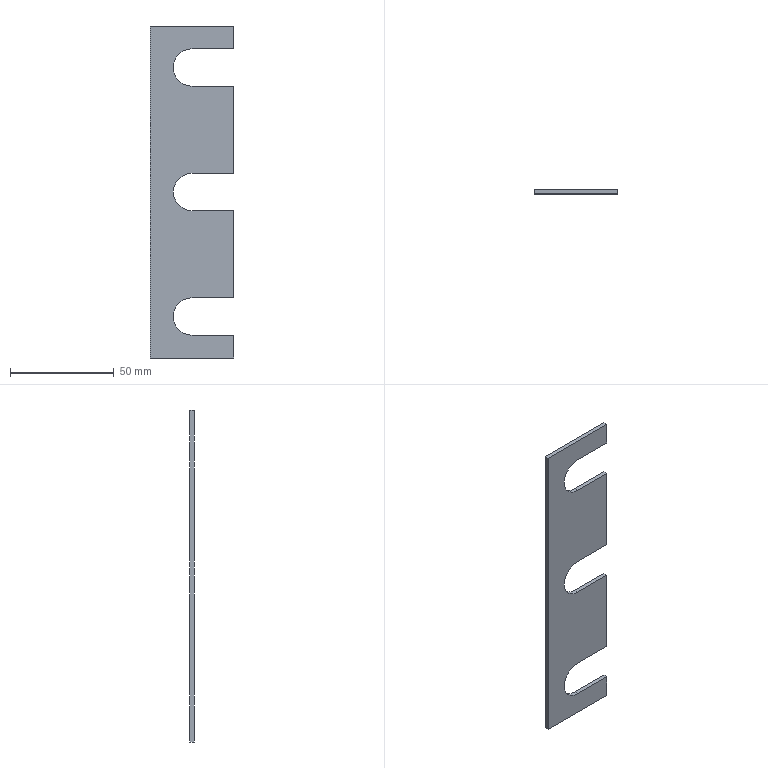Part | SolidWorks | features MirrorStock 1 | 1 solid | 18 faces | box 40 x 2 x 160 mm | volume 9877 mm3 | plane 15 | cylinder 3 | commonest cylinder face diameters 18 x3
STEP:
#1=CARTESIAN_POINT('',(0.,0.,-9.));
#2=VERTEX_POINT('',#1);
#3=CARTESIAN_POINT('',(0.,0.,9.));
#4=VERTEX_POINT('',#3);
#5=CARTESIAN_POINT('',(0.,0.,0.));
#6=DIRECTION('',(0.,1.,0.));
#7=DIRECTION('',(0.,0.,-1.));
#8=AXIS2_PLACEMENT_3D('',#5,#6,#7);
#9=CIRCLE('',#8,9.);
#10=EDGE_CURVE('',#2,#4,#9,.T.);
#11=ORIENTED_EDGE('',*,*,#10,.F.);
#12=CARTESIAN_POINT('',(0.,2.,-9.));
#13=VERTEX_POINT('',#12);
#14=CARTESIAN_POINT('',(0.,2.,-9.));
#15=DIRECTION('',(0.,-1.,0.));
#16=VECTOR('',#15,1000.);
#17=LINE('',#14,#16);
#18=EDGE_CURVE('',#13,#2,#17,.T.);
#19=ORIENTED_EDGE('',*,*,#18,.F.);
#20=CARTESIAN_POINT('',(0.,2.,9.));
#21=VERTEX_POINT('',#20);
#22=CARTESIAN_POINT('',(0.,2.,0.));
#23=DIRECTION('',(0.,1.,0.));
#24=DIRECTION('',(0.,0.,-1.));
#25=AXIS2_PLACEMENT_3D('',#22,#23,#24);
#26=CIRCLE('',#25,9.);
#27=EDGE_CURVE('',#13,#21,#26,.T.);
#28=ORIENTED_EDGE('',*,*,#27,.T.);
#29=CARTESIAN_POINT('',(0.,2.,9.));
#30=DIRECTION('',(0.,-1.,0.));
#31=VECTOR('',#30,1000.);
#32=LINE('',#29,#31);
#33=EDGE_CURVE('',#21,#4,#32,.T.);
#34=ORIENTED_EDGE('',*,*,#33,.T.);
#35=EDGE_LOOP('',(#11,#19,#28,#34));
#36=FACE_OUTER_BOUND('',#35,.T.);
#37=CARTESIAN_POINT('',(0.,2.,0.));
#38=DIRECTION('',(0.,-1.,0.));
#39=DIRECTION('',(0.,0.,1.));
#40=AXIS2_PLACEMENT_3D('',#37,#38,#39);
#41=CYLINDRICAL_SURFACE('',#40,9.);
#42=ADVANCED_FACE('',(#36),#41,.F.);
#43=CARTESIAN_POINT('',(20.,0.,9.));
#44=VERTEX_POINT('',#43);
#45=CARTESIAN_POINT('',(0.,0.,9.));
#46=DIRECTION('',(1.,0.,0.));
#47=VECTOR('',#46,1000.);
#48=LINE('',#45,#47);
#49=EDGE_CURVE('',#4,#44,#48,.T.);
#50=ORIENTED_EDGE('',*,*,#49,.F.);
#51=ORIENTED_EDGE('',*,*,#33,.F.);
#52=CARTESIAN_POINT('',(20.,2.,9.));
#53=VERTEX_POINT('',#52);
#54=CARTESIAN_POINT('',(0.,2.,9.));
#55=DIRECTION('',(1.,0.,0.));
#56=VECTOR('',#55,1000.);
#57=LINE('',#54,#56);
#58=EDGE_CURVE('',#21,#53,#57,.T.);
#59=ORIENTED_EDGE('',*,*,#58,.T.);
#60=CARTESIAN_POINT('',(20.,2.,9.));
#61=DIRECTION('',(0.,-1.,0.));
#62=VECTOR('',#61,1000.);
#63=LINE('',#60,#62);
#64=EDGE_CURVE('',#53,#44,#63,.T.);
#65=ORIENTED_EDGE('',*,*,#64,.T.);
#66=EDGE_LOOP('',(#50,#51,#59,#65));
#67=FACE_OUTER_BOUND('',#66,.T.);
#68=CARTESIAN_POINT('',(0.,2.,9.));
#69=DIRECTION('',(0.,0.,1.));
#70=DIRECTION('',(-1.,0.,0.));
#71=AXIS2_PLACEMENT_3D('',#68,#69,#70);
#72=PLANE('',#71);
#73=ADVANCED_FACE('',(#67),#72,.F.);
#74=CARTESIAN_POINT('',(20.,0.,51.));
#75=VERTEX_POINT('',#74);
#76=CARTESIAN_POINT('',(20.,0.,9.));
#77=DIRECTION('',(0.,0.,1.));
#78=VECTOR('',#77,1000.);
#79=LINE('',#76,#78);
#80=EDGE_CURVE('',#44,#75,#79,.T.);
#81=ORIENTED_EDGE('',*,*,#80,.F.);
#82=ORIENTED_EDGE('',*,*,#64,.F.);
#83=CARTESIAN_POINT('',(20.,2.,51.));
#84=VERTEX_POINT('',#83);
#85=CARTESIAN_POINT('',(20.,2.,9.));
#86=DIRECTION('',(0.,0.,1.));
#87=VECTOR('',#86,1000.);
#88=LINE('',#85,#87);
#89=EDGE_CURVE('',#53,#84,#88,.T.);
#90=ORIENTED_EDGE('',*,*,#89,.T.);
#91=CARTESIAN_POINT('',(20.,2.,51.));
#92=DIRECTION('',(0.,-1.,0.));
#93=VECTOR('',#92,1000.);
#94=LINE('',#91,#93);
#95=EDGE_CURVE('',#84,#75,#94,.T.);
#96=ORIENTED_EDGE('',*,*,#95,.T.);
#97=EDGE_LOOP('',(#81,#82,#90,#96));
#98=FACE_OUTER_BOUND('',#97,.T.);
#99=CARTESIAN_POINT('',(20.,2.,9.));
#100=DIRECTION('',(-1.,0.,0.));
#101=DIRECTION('',(0.,0.,-1.));
#102=AXIS2_PLACEMENT_3D('',#99,#100,#101);
#103=PLANE('',#102);
#104=ADVANCED_FACE('',(#98),#103,.F.);
#105=CARTESIAN_POINT('',(0.,0.,51.));
#106=VERTEX_POINT('',#105);
#107=CARTESIAN_POINT('',(20.,0.,51.));
#108=DIRECTION('',(-1.,0.,0.));
#109=VECTOR('',#108,1000.);
#110=LINE('',#107,#109);
#111=EDGE_CURVE('',#75,#106,#110,.T.);
#112=ORIENTED_EDGE('',*,*,#111,.F.);
#113=ORIENTED_EDGE('',*,*,#95,.F.);
#114=CARTESIAN_POINT('',(0.,2.,51.));
#115=VERTEX_POINT('',#114);
#116=CARTESIAN_POINT('',(20.,2.,51.));
#117=DIRECTION('',(-1.,0.,0.));
#118=VECTOR('',#117,1000.);
#119=LINE('',#116,#118);
#120=EDGE_CURVE('',#84,#115,#119,.T.);
#121=ORIENTED_EDGE('',*,*,#120,.T.);
#122=CARTESIAN_POINT('',(0.,2.,51.));
#123=DIRECTION('',(0.,-1.,0.));
#124=VECTOR('',#123,1000.);
#125=LINE('',#122,#124);
#126=EDGE_CURVE('',#115,#106,#125,.T.);
#127=ORIENTED_EDGE('',*,*,#126,.T.);
#128=EDGE_LOOP('',(#112,#113,#121,#127));
#129=FACE_OUTER_BOUND('',#128,.T.);
#130=CARTESIAN_POINT('',(20.,2.,51.));
#131=DIRECTION('',(0.,0.,-1.));
#132=DIRECTION('',(1.,0.,0.));
#133=AXIS2_PLACEMENT_3D('',#130,#131,#132);
#134=PLANE('',#133);
#135=ADVANCED_FACE('',(#129),#134,.F.);
#136=CARTESIAN_POINT('',(0.,0.,69.));
#137=VERTEX_POINT('',#136);
#138=CARTESIAN_POINT('',(0.,0.,60.));
#139=DIRECTION('',(0.,1.,0.));
#140=DIRECTION('',(0.,0.,1.));
#141=AXIS2_PLACEMENT_3D('',#138,#139,#140);
#142=CIRCLE('',#141,9.);
#143=EDGE_CURVE('',#106,#137,#142,.T.);
#144=ORIENTED_EDGE('',*,*,#143,.F.);
#145=ORIENTED_EDGE('',*,*,#126,.F.);
#146=CARTESIAN_POINT('',(0.,2.,69.));
#147=VERTEX_POINT('',#146);
#148=CARTESIAN_POINT('',(0.,2.,60.));
#149=DIRECTION('',(0.,1.,0.));
#150=DIRECTION('',(0.,0.,1.));
#151=AXIS2_PLACEMENT_3D('',#148,#149,#150);
#152=CIRCLE('',#151,9.);
#153=EDGE_CURVE('',#115,#147,#152,.T.);
#154=ORIENTED_EDGE('',*,*,#153,.T.);
#155=CARTESIAN_POINT('',(0.,2.,69.));
#156=DIRECTION('',(0.,-1.,0.));
#157=VECTOR('',#156,1000.);
#158=LINE('',#155,#157);
#159=EDGE_CURVE('',#147,#137,#158,.T.);
#160=ORIENTED_EDGE('',*,*,#159,.T.);
#161=EDGE_LOOP('',(#144,#145,#154,#160));
#162=FACE_OUTER_BOUND('',#161,.T.);
#163=CARTESIAN_POINT('',(0.,2.,60.));
#164=DIRECTION('',(0.,-1.,0.));
#165=DIRECTION('',(0.,0.,1.));
#166=AXIS2_PLACEMENT_3D('',#163,#164,#165);
#167=CYLINDRICAL_SURFACE('',#166,9.);
#168=ADVANCED_FACE('',(#162),#167,.F.);
#169=CARTESIAN_POINT('',(20.,0.,69.));
#170=VERTEX_POINT('',#169);
#171=CARTESIAN_POINT('',(0.,0.,69.));
#172=DIRECTION('',(1.,0.,0.));
#173=VECTOR('',#172,1000.);
#174=LINE('',#171,#173);
#175=EDGE_CURVE('',#137,#170,#174,.T.);
#176=ORIENTED_EDGE('',*,*,#175,.F.);
#177=ORIENTED_EDGE('',*,*,#159,.F.);
#178=CARTESIAN_POINT('',(20.,2.,69.));
#179=VERTEX_POINT('',#178);
#180=CARTESIAN_POINT('',(0.,2.,69.));
#181=DIRECTION('',(1.,0.,0.));
#182=VECTOR('',#181,1000.);
#183=LINE('',#180,#182);
#184=EDGE_CURVE('',#147,#179,#183,.T.);
#185=ORIENTED_EDGE('',*,*,#184,.T.);
#186=CARTESIAN_POINT('',(20.,2.,69.));
#187=DIRECTION('',(0.,-1.,0.));
#188=VECTOR('',#187,1000.);
#189=LINE('',#186,#188);
#190=EDGE_CURVE('',#179,#170,#189,.T.);
#191=ORIENTED_EDGE('',*,*,#190,.T.);
#192=EDGE_LOOP('',(#176,#177,#185,#191));
#193=FACE_OUTER_BOUND('',#192,.T.);
#194=CARTESIAN_POINT('',(0.,2.,69.));
#195=DIRECTION('',(0.,0.,1.));
#196=DIRECTION('',(-1.,0.,0.));
#197=AXIS2_PLACEMENT_3D('',#194,#195,#196);
#198=PLANE('',#197);
#199=ADVANCED_FACE('',(#193),#198,.F.);
#200=CARTESIAN_POINT('',(20.,0.,80.));
#201=VERTEX_POINT('',#200);
#202=CARTESIAN_POINT('',(20.,0.,69.));
#203=DIRECTION('',(0.,0.,1.));
#204=VECTOR('',#203,1000.);
#205=LINE('',#202,#204);
#206=EDGE_CURVE('',#170,#201,#205,.T.);
#207=ORIENTED_EDGE('',*,*,#206,.F.);
#208=ORIENTED_EDGE('',*,*,#190,.F.);
#209=CARTESIAN_POINT('',(20.,2.,80.));
#210=VERTEX_POINT('',#209);
#211=CARTESIAN_POINT('',(20.,2.,69.));
#212=DIRECTION('',(0.,0.,1.));
#213=VECTOR('',#212,1000.);
#214=LINE('',#211,#213);
#215=EDGE_CURVE('',#179,#210,#214,.T.);
#216=ORIENTED_EDGE('',*,*,#215,.T.);
#217=CARTESIAN_POINT('',(20.,2.,80.));
#218=DIRECTION('',(0.,-1.,0.));
#219=VECTOR('',#218,1000.);
#220=LINE('',#217,#219);
#221=EDGE_CURVE('',#210,#201,#220,.T.);
#222=ORIENTED_EDGE('',*,*,#221,.T.);
#223=EDGE_LOOP('',(#207,#208,#216,#222));
#224=FACE_OUTER_BOUND('',#223,.T.);
#225=CARTESIAN_POINT('',(20.,2.,69.));
#226=DIRECTION('',(-1.,0.,0.));
#227=DIRECTION('',(0.,0.,-1.));
#228=AXIS2_PLACEMENT_3D('',#225,#226,#227);
#229=PLANE('',#228);
#230=ADVANCED_FACE('',(#224),#229,.F.);
#231=CARTESIAN_POINT('',(-20.,0.,80.));
#232=VERTEX_POINT('',#231);
#233=CARTESIAN_POINT('',(20.,0.,80.));
#234=DIRECTION('',(-1.,0.,0.));
#235=VECTOR('',#234,1000.);
#236=LINE('',#233,#235);
#237=EDGE_CURVE('',#201,#232,#236,.T.);
#238=ORIENTED_EDGE('',*,*,#237,.F.);
#239=ORIENTED_EDGE('',*,*,#221,.F.);
#240=CARTESIAN_POINT('',(-20.,2.,80.));
#241=VERTEX_POINT('',#240);
#242=CARTESIAN_POINT('',(20.,2.,80.));
#243=DIRECTION('',(-1.,0.,0.));
#244=VECTOR('',#243,1000.);
#245=LINE('',#242,#244);
#246=EDGE_CURVE('',#210,#241,#245,.T.);
#247=ORIENTED_EDGE('',*,*,#246,.T.);
#248=CARTESIAN_POINT('',(-20.,2.,80.));
#249=DIRECTION('',(0.,-1.,0.));
#250=VECTOR('',#249,1000.);
#251=LINE('',#248,#250);
#252=EDGE_CURVE('',#241,#232,#251,.T.);
#253=ORIENTED_EDGE('',*,*,#252,.T.);
#254=EDGE_LOOP('',(#238,#239,#247,#253));
#255=FACE_OUTER_BOUND('',#254,.T.);
#256=CARTESIAN_POINT('',(20.,2.,80.));
#257=DIRECTION('',(0.,0.,-1.));
#258=DIRECTION('',(1.,0.,0.));
#259=AXIS2_PLACEMENT_3D('',#256,#257,#258);
#260=PLANE('',#259);
#261=ADVANCED_FACE('',(#255),#260,.F.);
#262=CARTESIAN_POINT('',(-20.,0.,-80.));
#263=VERTEX_POINT('',#262);
#264=CARTESIAN_POINT('',(-20.,0.,80.));
#265=DIRECTION('',(0.,0.,-1.));
#266=VECTOR('',#265,1000.);
#267=LINE('',#264,#266);
#268=EDGE_CURVE('',#232,#263,#267,.T.);
#269=ORIENTED_EDGE('',*,*,#268,.F.);
#270=ORIENTED_EDGE('',*,*,#252,.F.);
#271=CARTESIAN_POINT('',(-20.,2.,-80.));
#272=VERTEX_POINT('',#271);
#273=CARTESIAN_POINT('',(-20.,2.,80.));
#274=DIRECTION('',(0.,0.,-1.));
#275=VECTOR('',#274,1000.);
#276=LINE('',#273,#275);
#277=EDGE_CURVE('',#241,#272,#276,.T.);
#278=ORIENTED_EDGE('',*,*,#277,.T.);
#279=CARTESIAN_POINT('',(-20.,2.,-80.));
#280=DIRECTION('',(0.,-1.,0.));
#281=VECTOR('',#280,1000.);
#282=LINE('',#279,#281);
#283=EDGE_CURVE('',#272,#263,#282,.T.);
#284=ORIENTED_EDGE('',*,*,#283,.T.);
#285=EDGE_LOOP('',(#269,#270,#278,#284));
#286=FACE_OUTER_BOUND('',#285,.T.);
#287=CARTESIAN_POINT('',(-20.,2.,80.));
#288=DIRECTION('',(1.,0.,0.));
#289=DIRECTION('',(0.,0.,1.));
#290=AXIS2_PLACEMENT_3D('',#287,#288,#289);
#291=PLANE('',#290);
#292=ADVANCED_FACE('',(#286),#291,.F.);
#293=CARTESIAN_POINT('',(20.,0.,-80.));
#294=VERTEX_POINT('',#293);
#295=CARTESIAN_POINT('',(20.,0.,-80.));
#296=DIRECTION('',(1.,0.,0.));
#297=VECTOR('',#296,1000.);
#298=LINE('',#295,#297);
#299=EDGE_CURVE('',#263,#294,#298,.T.);
#300=ORIENTED_EDGE('',*,*,#299,.F.);
#301=ORIENTED_EDGE('',*,*,#283,.F.);
#302=CARTESIAN_POINT('',(20.,2.,-80.));
#303=VERTEX_POINT('',#302);
#304=CARTESIAN_POINT('',(20.,2.,-80.));
#305=DIRECTION('',(1.,0.,0.));
#306=VECTOR('',#305,1000.);
#307=LINE('',#304,#306);
#308=EDGE_CURVE('',#272,#303,#307,.T.);
#309=ORIENTED_EDGE('',*,*,#308,.T.);
#310=CARTESIAN_POINT('',(20.,2.,-80.));
#311=DIRECTION('',(0.,-1.,0.));
#312=VECTOR('',#311,1000.);
#313=LINE('',#310,#312);
#314=EDGE_CURVE('',#303,#294,#313,.T.);
#315=ORIENTED_EDGE('',*,*,#314,.T.);
#316=EDGE_LOOP('',(#300,#301,#309,#315));
#317=FACE_OUTER_BOUND('',#316,.T.);
#318=CARTESIAN_POINT('',(20.,2.,-80.));
#319=DIRECTION('',(0.,0.,1.));
#320=DIRECTION('',(-1.,0.,0.));
#321=AXIS2_PLACEMENT_3D('',#318,#319,#320);
#322=PLANE('',#321);
#323=ADVANCED_FACE('',(#317),#322,.F.);
#324=CARTESIAN_POINT('',(20.,0.,-69.));
#325=VERTEX_POINT('',#324);
#326=CARTESIAN_POINT('',(20.,0.,-69.));
#327=DIRECTION('',(0.,0.,1.));
#328=VECTOR('',#327,1000.);
#329=LINE('',#326,#328);
#330=EDGE_CURVE('',#294,#325,#329,.T.);
#331=ORIENTED_EDGE('',*,*,#330,.F.);
#332=ORIENTED_EDGE('',*,*,#314,.F.);
#333=CARTESIAN_POINT('',(20.,2.,-69.));
#334=VERTEX_POINT('',#333);
#335=CARTESIAN_POINT('',(20.,2.,-69.));
#336=DIRECTION('',(0.,0.,1.));
#337=VECTOR('',#336,1000.);
#338=LINE('',#335,#337);
#339=EDGE_CURVE('',#303,#334,#338,.T.);
#340=ORIENTED_EDGE('',*,*,#339,.T.);
#341=CARTESIAN_POINT('',(20.,2.,-69.));
#342=DIRECTION('',(0.,-1.,0.));
#343=VECTOR('',#342,1000.);
#344=LINE('',#341,#343);
#345=EDGE_CURVE('',#334,#325,#344,.T.);
#346=ORIENTED_EDGE('',*,*,#345,.T.);
#347=EDGE_LOOP('',(#331,#332,#340,#346));
#348=FACE_OUTER_BOUND('',#347,.T.);
#349=CARTESIAN_POINT('',(20.,2.,-69.));
#350=DIRECTION('',(-1.,0.,0.));
#351=DIRECTION('',(0.,0.,-1.));
#352=AXIS2_PLACEMENT_3D('',#349,#350,#351);
#353=PLANE('',#352);
#354=ADVANCED_FACE('',(#348),#353,.F.);
#355=CARTESIAN_POINT('',(0.,0.,-69.));
#356=VERTEX_POINT('',#355);
#357=CARTESIAN_POINT('',(0.,0.,-69.));
#358=DIRECTION('',(-1.,0.,0.));
#359=VECTOR('',#358,1000.);
#360=LINE('',#357,#359);
#361=EDGE_CURVE('',#325,#356,#360,.T.);
#362=ORIENTED_EDGE('',*,*,#361,.F.);
#363=ORIENTED_EDGE('',*,*,#345,.F.);
#364=CARTESIAN_POINT('',(0.,2.,-69.));
#365=VERTEX_POINT('',#364);
#366=CARTESIAN_POINT('',(0.,2.,-69.));
#367=DIRECTION('',(-1.,0.,0.));
#368=VECTOR('',#367,1000.);
#369=LINE('',#366,#368);
#370=EDGE_CURVE('',#334,#365,#369,.T.);
#371=ORIENTED_EDGE('',*,*,#370,.T.);
#372=CARTESIAN_POINT('',(0.,2.,-69.));
#373=DIRECTION('',(0.,-1.,0.));
#374=VECTOR('',#373,1000.);
#375=LINE('',#372,#374);
#376=EDGE_CURVE('',#365,#356,#375,.T.);
#377=ORIENTED_EDGE('',*,*,#376,.T.);
#378=EDGE_LOOP('',(#362,#363,#371,#377));
#379=FACE_OUTER_BOUND('',#378,.T.);
#380=CARTESIAN_POINT('',(0.,2.,-69.));
#381=DIRECTION('',(0.,0.,-1.));
#382=DIRECTION('',(1.,0.,0.));
#383=AXIS2_PLACEMENT_3D('',#380,#381,#382);
#384=PLANE('',#383);
#385=ADVANCED_FACE('',(#379),#384,.F.);
#386=CARTESIAN_POINT('',(0.,0.,-51.));
#387=VERTEX_POINT('',#386);
#388=CARTESIAN_POINT('',(0.,0.,-60.));
#389=DIRECTION('',(0.,1.,0.));
#390=DIRECTION('',(0.,0.,-1.));
#391=AXIS2_PLACEMENT_3D('',#388,#389,#390);
#392=CIRCLE('',#391,9.);
#393=EDGE_CURVE('',#356,#387,#392,.T.);
#394=ORIENTED_EDGE('',*,*,#393,.F.);
#395=ORIENTED_EDGE('',*,*,#376,.F.);
#396=CARTESIAN_POINT('',(0.,2.,-51.));
#397=VERTEX_POINT('',#396);
#398=CARTESIAN_POINT('',(0.,2.,-60.));
#399=DIRECTION('',(0.,1.,0.));
#400=DIRECTION('',(0.,0.,-1.));
#401=AXIS2_PLACEMENT_3D('',#398,#399,#400);
#402=CIRCLE('',#401,9.);
#403=EDGE_CURVE('',#365,#397,#402,.T.);
#404=ORIENTED_EDGE('',*,*,#403,.T.);
#405=CARTESIAN_POINT('',(0.,2.,-51.));
#406=DIRECTION('',(0.,-1.,0.));
#407=VECTOR('',#406,1000.);
#408=LINE('',#405,#407);
#409=EDGE_CURVE('',#397,#387,#408,.T.);
#410=ORIENTED_EDGE('',*,*,#409,.T.);
#411=EDGE_LOOP('',(#394,#395,#404,#410));
#412=FACE_OUTER_BOUND('',#411,.T.);
#413=CARTESIAN_POINT('',(0.,2.,-60.));
#414=DIRECTION('',(0.,-1.,0.));
#415=DIRECTION('',(0.,0.,1.));
#416=AXIS2_PLACEMENT_3D('',#413,#414,#415);
#417=CYLINDRICAL_SURFACE('',#416,9.);
#418=ADVANCED_FACE('',(#412),#417,.F.);
#419=CARTESIAN_POINT('',(20.,0.,-51.));
#420=VERTEX_POINT('',#419);
#421=CARTESIAN_POINT('',(20.,0.,-51.));
#422=DIRECTION('',(1.,0.,0.));
#423=VECTOR('',#422,1000.);
#424=LINE('',#421,#423);
#425=EDGE_CURVE('',#387,#420,#424,.T.);
#426=ORIENTED_EDGE('',*,*,#425,.F.);
#427=ORIENTED_EDGE('',*,*,#409,.F.);
#428=CARTESIAN_POINT('',(20.,2.,-51.));
#429=VERTEX_POINT('',#428);
#430=CARTESIAN_POINT('',(20.,2.,-51.));
#431=DIRECTION('',(1.,0.,0.));
#432=VECTOR('',#431,1000.);
#433=LINE('',#430,#432);
#434=EDGE_CURVE('',#397,#429,#433,.T.);
#435=ORIENTED_EDGE('',*,*,#434,.T.);
#436=CARTESIAN_POINT('',(20.,2.,-51.));
#437=DIRECTION('',(0.,-1.,0.));
#438=VECTOR('',#437,1000.);
#439=LINE('',#436,#438);
#440=EDGE_CURVE('',#429,#420,#439,.T.);
#441=ORIENTED_EDGE('',*,*,#440,.T.);
#442=EDGE_LOOP('',(#426,#427,#435,#441));
#443=FACE_OUTER_BOUND('',#442,.T.);
#444=CARTESIAN_POINT('',(20.,2.,-51.));
#445=DIRECTION('',(0.,0.,1.));
#446=DIRECTION('',(-1.,0.,0.));
#447=AXIS2_PLACEMENT_3D('',#444,#445,#446);
#448=PLANE('',#447);
#449=ADVANCED_FACE('',(#443),#448,.F.);
#450=CARTESIAN_POINT('',(20.,0.,-9.));
#451=VERTEX_POINT('',#450);
#452=CARTESIAN_POINT('',(20.,0.,-9.));
#453=DIRECTION('',(0.,0.,1.));
#454=VECTOR('',#453,1000.);
#455=LINE('',#452,#454);
#456=EDGE_CURVE('',#420,#451,#455,.T.);
#457=ORIENTED_EDGE('',*,*,#456,.F.);
#458=ORIENTED_EDGE('',*,*,#440,.F.);
#459=CARTESIAN_POINT('',(20.,2.,-9.));
#460=VERTEX_POINT('',#459);
#461=CARTESIAN_POINT('',(20.,2.,-9.));
#462=DIRECTION('',(0.,0.,1.));
#463=VECTOR('',#462,1000.);
#464=LINE('',#461,#463);
#465=EDGE_CURVE('',#429,#460,#464,.T.);
#466=ORIENTED_EDGE('',*,*,#465,.T.);
#467=CARTESIAN_POINT('',(20.,2.,-9.));
#468=DIRECTION('',(0.,-1.,0.));
#469=VECTOR('',#468,1000.);
#470=LINE('',#467,#469);
#471=EDGE_CURVE('',#460,#451,#470,.T.);
#472=ORIENTED_EDGE('',*,*,#471,.T.);
#473=EDGE_LOOP('',(#457,#458,#466,#472));
#474=FACE_OUTER_BOUND('',#473,.T.);
#475=CARTESIAN_POINT('',(20.,2.,-9.));
#476=DIRECTION('',(-1.,0.,0.));
#477=DIRECTION('',(0.,0.,-1.));
#478=AXIS2_PLACEMENT_3D('',#475,#476,#477);
#479=PLANE('',#478);
#480=ADVANCED_FACE('',(#474),#479,.F.);
#481=CARTESIAN_POINT('',(0.,0.,-9.));
#482=DIRECTION('',(-1.,0.,0.));
#483=VECTOR('',#482,1000.);
#484=LINE('',#481,#483);
#485=EDGE_CURVE('',#451,#2,#484,.T.);
#486=ORIENTED_EDGE('',*,*,#485,.F.);
#487=ORIENTED_EDGE('',*,*,#471,.F.);
#488=CARTESIAN_POINT('',(0.,2.,-9.));
#489=DIRECTION('',(-1.,0.,0.));
#490=VECTOR('',#489,1000.);
#491=LINE('',#488,#490);
#492=EDGE_CURVE('',#460,#13,#491,.T.);
#493=ORIENTED_EDGE('',*,*,#492,.T.);
#494=ORIENTED_EDGE('',*,*,#18,.T.);
#495=EDGE_LOOP('',(#486,#487,#493,#494));
#496=FACE_OUTER_BOUND('',#495,.T.);
#497=CARTESIAN_POINT('',(0.,2.,-9.));
#498=DIRECTION('',(0.,0.,-1.));
#499=DIRECTION('',(1.,0.,0.));
#500=AXIS2_PLACEMENT_3D('',#497,#498,#499);
#501=PLANE('',#500);
#502=ADVANCED_FACE('',(#496),#501,.F.);
#503=ORIENTED_EDGE('',*,*,#27,.F.);
#504=ORIENTED_EDGE('',*,*,#492,.F.);
#505=ORIENTED_EDGE('',*,*,#465,.F.);
#506=ORIENTED_EDGE('',*,*,#434,.F.);
#507=ORIENTED_EDGE('',*,*,#403,.F.);
#508=ORIENTED_EDGE('',*,*,#370,.F.);
#509=ORIENTED_EDGE('',*,*,#339,.F.);
#510=ORIENTED_EDGE('',*,*,#308,.F.);
#511=ORIENTED_EDGE('',*,*,#277,.F.);
#512=ORIENTED_EDGE('',*,*,#246,.F.);
#513=ORIENTED_EDGE('',*,*,#215,.F.);
#514=ORIENTED_EDGE('',*,*,#184,.F.);
#515=ORIENTED_EDGE('',*,*,#153,.F.);
#516=ORIENTED_EDGE('',*,*,#120,.F.);
#517=ORIENTED_EDGE('',*,*,#89,.F.);
#518=ORIENTED_EDGE('',*,*,#58,.F.);
#519=EDGE_LOOP('',(#503,#504,#505,#506,#507,#508,#509,#510,#511,#512,#513,#514,#515,#516,#517,#518));
#520=FACE_OUTER_BOUND('',#519,.T.);
#521=CARTESIAN_POINT('',(0.,2.,0.));
#522=DIRECTION('',(0.,1.,0.));
#523=DIRECTION('',(0.,0.,-1.));
#524=AXIS2_PLACEMENT_3D('',#521,#522,#523);
#525=PLANE('',#524);
#526=ADVANCED_FACE('',(#520),#525,.T.);
#527=ORIENTED_EDGE('',*,*,#10,.T.);
#528=ORIENTED_EDGE('',*,*,#49,.T.);
#529=ORIENTED_EDGE('',*,*,#80,.T.);
#530=ORIENTED_EDGE('',*,*,#111,.T.);
#531=ORIENTED_EDGE('',*,*,#143,.T.);
#532=ORIENTED_EDGE('',*,*,#175,.T.);
#533=ORIENTED_EDGE('',*,*,#206,.T.);
#534=ORIENTED_EDGE('',*,*,#237,.T.);
#535=ORIENTED_EDGE('',*,*,#268,.T.);
#536=ORIENTED_EDGE('',*,*,#299,.T.);
#537=ORIENTED_EDGE('',*,*,#330,.T.);
#538=ORIENTED_EDGE('',*,*,#361,.T.);
#539=ORIENTED_EDGE('',*,*,#393,.T.);
#540=ORIENTED_EDGE('',*,*,#425,.T.);
#541=ORIENTED_EDGE('',*,*,#456,.T.);
#542=ORIENTED_EDGE('',*,*,#485,.T.);
#543=EDGE_LOOP('',(#527,#528,#529,#530,#531,#532,#533,#534,#535,#536,#537,#538,#539,#540,#541,#542));
#544=FACE_OUTER_BOUND('',#543,.T.);
#545=CARTESIAN_POINT('',(0.,0.,0.));
#546=DIRECTION('',(0.,1.,0.));
#547=DIRECTION('',(0.,0.,-1.));
#548=AXIS2_PLACEMENT_3D('',#545,#546,#547);
#549=PLANE('',#548);
#550=ADVANCED_FACE('',(#544),#549,.F.);
#551=CLOSED_SHELL('',(#42,#73,#104,#135,#168,#199,#230,#261,#292,#323,#354,#385,#418,#449,#480,#502,#526,#550));
#552=MANIFOLD_SOLID_BREP('',#551);
#553=CARTESIAN_POINT('',(0.,0.,0.));
#554=DIRECTION('',(0.,0.,1.));
#555=DIRECTION('',(1.,0.,0.));
#556=AXIS2_PLACEMENT_3D('',#553,#554,#555);
#557=(LENGTH_UNIT()NAMED_UNIT(*)SI_UNIT(.MILLI.,.METRE.));
#558=UNCERTAINTY_MEASURE_WITH_UNIT(LENGTH_MEASURE(0.00001),#557,'','');
#559=(NAMED_UNIT(*)PLANE_ANGLE_UNIT()SI_UNIT($,.RADIAN.));
#560=(NAMED_UNIT(*)SI_UNIT($,.STERADIAN.)SOLID_ANGLE_UNIT());
#561=(GEOMETRIC_REPRESENTATION_CONTEXT(3)GLOBAL_UNCERTAINTY_ASSIGNED_CONTEXT((#558))GLOBAL_UNIT_ASSIGNED_CONTEXT((#557,#559,#560))REPRESENTATION_CONTEXT('',''));
#562=ADVANCED_BREP_SHAPE_REPRESENTATION('',(#552,#556),#561);